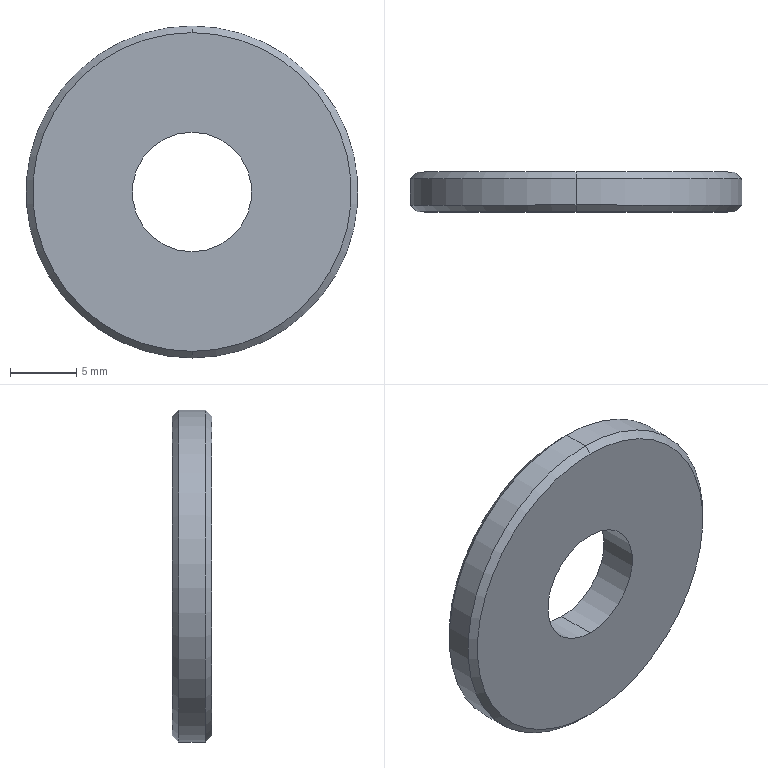Part | SolidWorks | features Chamfer 1, Extrusion 1, ICE 1 | 1 solid | 10 faces | box 25 x 3 x 25 mm | volume 1262 mm3 | cone 4 | cylinder 4 | plane 2 | commonest cylinder face diameters 9 x2 25 x2
STEP:
#1=CARTESIAN_POINT('',(0.,3.,12.));
#2=VERTEX_POINT('',#1);
#3=CARTESIAN_POINT('',(0.,3.,-12.));
#4=VERTEX_POINT('',#3);
#5=CARTESIAN_POINT('',(0.,3.,0.));
#6=DIRECTION('',(0.,1.,0.));
#7=DIRECTION('',(0.,0.,1.));
#8=AXIS2_PLACEMENT_3D('',#5,#6,#7);
#9=CIRCLE('',#8,12.);
#10=EDGE_CURVE('',#2,#4,#9,.T.);
#11=ORIENTED_EDGE('',*,*,#10,.F.);
#12=CARTESIAN_POINT('',(0.,2.5,12.5));
#13=VERTEX_POINT('',#12);
#14=CARTESIAN_POINT('',(0.,3.,12.));
#15=DIRECTION('',(0.,-0.7071,0.7071));
#16=VECTOR('',#15,1000.);
#17=LINE('',#14,#16);
#18=EDGE_CURVE('',#2,#13,#17,.T.);
#19=ORIENTED_EDGE('',*,*,#18,.T.);
#20=CARTESIAN_POINT('',(0.,2.5,-12.5));
#21=VERTEX_POINT('',#20);
#22=CARTESIAN_POINT('',(0.,2.5,0.));
#23=DIRECTION('',(0.,-1.,0.));
#24=DIRECTION('',(0.,0.,1.));
#25=AXIS2_PLACEMENT_3D('',#22,#23,#24);
#26=CIRCLE('',#25,12.5);
#27=EDGE_CURVE('',#21,#13,#26,.T.);
#28=ORIENTED_EDGE('',*,*,#27,.F.);
#29=CARTESIAN_POINT('',(0.,3.,-12.));
#30=DIRECTION('',(0.,-0.7071,-0.7071));
#31=VECTOR('',#30,1000.);
#32=LINE('',#29,#31);
#33=EDGE_CURVE('',#4,#21,#32,.T.);
#34=ORIENTED_EDGE('',*,*,#33,.F.);
#35=EDGE_LOOP('',(#11,#19,#28,#34));
#36=FACE_OUTER_BOUND('',#35,.T.);
#37=CARTESIAN_POINT('',(0.,3.,0.));
#38=DIRECTION('',(0.,-1.,0.));
#39=DIRECTION('',(0.,0.,-1.));
#40=AXIS2_PLACEMENT_3D('',#37,#38,#39);
#41=CONICAL_SURFACE('',#40,12.,0.7854);
#42=ADVANCED_FACE('',(#36),#41,.T.);
#43=CARTESIAN_POINT('',(0.,0.,-12.));
#44=VERTEX_POINT('',#43);
#45=CARTESIAN_POINT('',(0.,0.,12.));
#46=VERTEX_POINT('',#45);
#47=CARTESIAN_POINT('',(0.,0.,0.));
#48=DIRECTION('',(0.,-1.,0.));
#49=DIRECTION('',(0.,0.,1.));
#50=AXIS2_PLACEMENT_3D('',#47,#48,#49);
#51=CIRCLE('',#50,12.);
#52=EDGE_CURVE('',#44,#46,#51,.T.);
#53=ORIENTED_EDGE('',*,*,#52,.F.);
#54=CARTESIAN_POINT('',(0.,0.5,-12.5));
#55=VERTEX_POINT('',#54);
#56=CARTESIAN_POINT('',(0.,0.5,-12.5));
#57=DIRECTION('',(0.,0.7071,-0.7071));
#58=VECTOR('',#57,1000.);
#59=LINE('',#56,#58);
#60=EDGE_CURVE('',#44,#55,#59,.T.);
#61=ORIENTED_EDGE('',*,*,#60,.T.);
#62=CARTESIAN_POINT('',(0.,0.5,12.5));
#63=VERTEX_POINT('',#62);
#64=CARTESIAN_POINT('',(0.,0.5,0.));
#65=DIRECTION('',(0.,1.,0.));
#66=DIRECTION('',(0.,0.,1.));
#67=AXIS2_PLACEMENT_3D('',#64,#65,#66);
#68=CIRCLE('',#67,12.5);
#69=EDGE_CURVE('',#63,#55,#68,.T.);
#70=ORIENTED_EDGE('',*,*,#69,.F.);
#71=CARTESIAN_POINT('',(0.,0.5,12.5));
#72=DIRECTION('',(0.,0.7071,0.7071));
#73=VECTOR('',#72,1000.);
#74=LINE('',#71,#73);
#75=EDGE_CURVE('',#46,#63,#74,.T.);
#76=ORIENTED_EDGE('',*,*,#75,.F.);
#77=EDGE_LOOP('',(#53,#61,#70,#76));
#78=FACE_OUTER_BOUND('',#77,.T.);
#79=CARTESIAN_POINT('',(0.,0.5,0.));
#80=DIRECTION('',(0.,1.,0.));
#81=DIRECTION('',(0.,0.,1.));
#82=AXIS2_PLACEMENT_3D('',#79,#80,#81);
#83=CONICAL_SURFACE('',#82,12.5,0.7854);
#84=ADVANCED_FACE('',(#78),#83,.T.);
#85=CARTESIAN_POINT('',(0.,0.,-4.5));
#86=VERTEX_POINT('',#85);
#87=CARTESIAN_POINT('',(0.,0.,4.5));
#88=VERTEX_POINT('',#87);
#89=CARTESIAN_POINT('',(0.,0.,0.));
#90=DIRECTION('',(0.,1.,0.));
#91=DIRECTION('',(0.,0.,1.));
#92=AXIS2_PLACEMENT_3D('',#89,#90,#91);
#93=CIRCLE('',#92,4.5);
#94=EDGE_CURVE('',#86,#88,#93,.T.);
#95=ORIENTED_EDGE('',*,*,#94,.F.);
#96=CARTESIAN_POINT('',(0.,3.,-4.5));
#97=VERTEX_POINT('',#96);
#98=CARTESIAN_POINT('',(0.,0.,-4.5));
#99=DIRECTION('',(0.,1.,0.));
#100=VECTOR('',#99,1000.);
#101=LINE('',#98,#100);
#102=EDGE_CURVE('',#86,#97,#101,.T.);
#103=ORIENTED_EDGE('',*,*,#102,.T.);
#104=CARTESIAN_POINT('',(0.,3.,4.5));
#105=VERTEX_POINT('',#104);
#106=CARTESIAN_POINT('',(0.,3.,0.));
#107=DIRECTION('',(0.,1.,0.));
#108=DIRECTION('',(0.,0.,1.));
#109=AXIS2_PLACEMENT_3D('',#106,#107,#108);
#110=CIRCLE('',#109,4.5);
#111=EDGE_CURVE('',#97,#105,#110,.T.);
#112=ORIENTED_EDGE('',*,*,#111,.T.);
#113=CARTESIAN_POINT('',(0.,0.,4.5));
#114=DIRECTION('',(0.,1.,0.));
#115=VECTOR('',#114,1000.);
#116=LINE('',#113,#115);
#117=EDGE_CURVE('',#88,#105,#116,.T.);
#118=ORIENTED_EDGE('',*,*,#117,.F.);
#119=EDGE_LOOP('',(#95,#103,#112,#118));
#120=FACE_OUTER_BOUND('',#119,.T.);
#121=CARTESIAN_POINT('',(0.,0.,0.));
#122=DIRECTION('',(0.,1.,0.));
#123=DIRECTION('',(0.,0.,1.));
#124=AXIS2_PLACEMENT_3D('',#121,#122,#123);
#125=CYLINDRICAL_SURFACE('',#124,4.5);
#126=ADVANCED_FACE('',(#120),#125,.F.);
#127=ORIENTED_EDGE('',*,*,#27,.T.);
#128=CARTESIAN_POINT('',(0.,3.,12.5));
#129=DIRECTION('',(0.,-1.,0.));
#130=VECTOR('',#129,1000.);
#131=LINE('',#128,#130);
#132=EDGE_CURVE('',#13,#63,#131,.T.);
#133=ORIENTED_EDGE('',*,*,#132,.T.);
#134=ORIENTED_EDGE('',*,*,#69,.T.);
#135=CARTESIAN_POINT('',(0.,3.,-12.5));
#136=DIRECTION('',(0.,-1.,0.));
#137=VECTOR('',#136,1000.);
#138=LINE('',#135,#137);
#139=EDGE_CURVE('',#21,#55,#138,.T.);
#140=ORIENTED_EDGE('',*,*,#139,.F.);
#141=EDGE_LOOP('',(#127,#133,#134,#140));
#142=FACE_OUTER_BOUND('',#141,.T.);
#143=CARTESIAN_POINT('',(0.,3.,0.));
#144=DIRECTION('',(0.,-1.,0.));
#145=DIRECTION('',(0.,0.,-1.));
#146=AXIS2_PLACEMENT_3D('',#143,#144,#145);
#147=CYLINDRICAL_SURFACE('',#146,12.5);
#148=ADVANCED_FACE('',(#142),#147,.T.);
#149=ORIENTED_EDGE('',*,*,#132,.F.);
#150=CARTESIAN_POINT('',(0.,2.5,0.));
#151=DIRECTION('',(0.,-1.,0.));
#152=DIRECTION('',(0.,0.,1.));
#153=AXIS2_PLACEMENT_3D('',#150,#151,#152);
#154=CIRCLE('',#153,12.5);
#155=EDGE_CURVE('',#13,#21,#154,.T.);
#156=ORIENTED_EDGE('',*,*,#155,.T.);
#157=ORIENTED_EDGE('',*,*,#139,.T.);
#158=CARTESIAN_POINT('',(0.,0.5,0.));
#159=DIRECTION('',(0.,1.,0.));
#160=DIRECTION('',(0.,0.,1.));
#161=AXIS2_PLACEMENT_3D('',#158,#159,#160);
#162=CIRCLE('',#161,12.5);
#163=EDGE_CURVE('',#55,#63,#162,.T.);
#164=ORIENTED_EDGE('',*,*,#163,.T.);
#165=EDGE_LOOP('',(#149,#156,#157,#164));
#166=FACE_OUTER_BOUND('',#165,.T.);
#167=CARTESIAN_POINT('',(0.,3.,0.));
#168=DIRECTION('',(0.,-1.,0.));
#169=DIRECTION('',(0.,0.,-1.));
#170=AXIS2_PLACEMENT_3D('',#167,#168,#169);
#171=CYLINDRICAL_SURFACE('',#170,12.5);
#172=ADVANCED_FACE('',(#166),#171,.T.);
#173=CARTESIAN_POINT('',(0.,3.,0.));
#174=DIRECTION('',(0.,1.,0.));
#175=DIRECTION('',(0.,0.,1.));
#176=AXIS2_PLACEMENT_3D('',#173,#174,#175);
#177=CIRCLE('',#176,12.);
#178=EDGE_CURVE('',#4,#2,#177,.T.);
#179=ORIENTED_EDGE('',*,*,#178,.T.);
#180=ORIENTED_EDGE('',*,*,#10,.T.);
#181=EDGE_LOOP('',(#179,#180));
#182=FACE_OUTER_BOUND('',#181,.T.);
#183=CARTESIAN_POINT('',(0.,3.,0.));
#184=DIRECTION('',(0.,1.,0.));
#185=DIRECTION('',(0.,0.,1.));
#186=AXIS2_PLACEMENT_3D('',#183,#184,#185);
#187=CIRCLE('',#186,4.5);
#188=EDGE_CURVE('',#105,#97,#187,.T.);
#189=ORIENTED_EDGE('',*,*,#188,.F.);
#190=ORIENTED_EDGE('',*,*,#111,.F.);
#191=EDGE_LOOP('',(#189,#190));
#192=FACE_BOUND('',#191,.T.);
#193=CARTESIAN_POINT('',(0.,3.,0.));
#194=DIRECTION('',(0.,1.,0.));
#195=DIRECTION('',(0.,0.,1.));
#196=AXIS2_PLACEMENT_3D('',#193,#194,#195);
#197=PLANE('',#196);
#198=ADVANCED_FACE('',(#182,#192),#197,.T.);
#199=CARTESIAN_POINT('',(0.,0.,0.));
#200=DIRECTION('',(0.,-1.,0.));
#201=DIRECTION('',(0.,0.,1.));
#202=AXIS2_PLACEMENT_3D('',#199,#200,#201);
#203=CIRCLE('',#202,12.);
#204=EDGE_CURVE('',#46,#44,#203,.T.);
#205=ORIENTED_EDGE('',*,*,#204,.T.);
#206=ORIENTED_EDGE('',*,*,#52,.T.);
#207=EDGE_LOOP('',(#205,#206));
#208=FACE_OUTER_BOUND('',#207,.T.);
#209=CARTESIAN_POINT('',(0.,0.,0.));
#210=DIRECTION('',(0.,1.,0.));
#211=DIRECTION('',(0.,0.,1.));
#212=AXIS2_PLACEMENT_3D('',#209,#210,#211);
#213=CIRCLE('',#212,4.5);
#214=EDGE_CURVE('',#88,#86,#213,.T.);
#215=ORIENTED_EDGE('',*,*,#214,.T.);
#216=ORIENTED_EDGE('',*,*,#94,.T.);
#217=EDGE_LOOP('',(#215,#216));
#218=FACE_BOUND('',#217,.T.);
#219=CARTESIAN_POINT('',(0.,0.,0.));
#220=DIRECTION('',(0.,1.,0.));
#221=DIRECTION('',(0.,0.,1.));
#222=AXIS2_PLACEMENT_3D('',#219,#220,#221);
#223=PLANE('',#222);
#224=ADVANCED_FACE('',(#208,#218),#223,.F.);
#225=ORIENTED_EDGE('',*,*,#102,.F.);
#226=ORIENTED_EDGE('',*,*,#214,.F.);
#227=ORIENTED_EDGE('',*,*,#117,.T.);
#228=ORIENTED_EDGE('',*,*,#188,.T.);
#229=EDGE_LOOP('',(#225,#226,#227,#228));
#230=FACE_OUTER_BOUND('',#229,.T.);
#231=CARTESIAN_POINT('',(0.,0.,0.));
#232=DIRECTION('',(0.,1.,0.));
#233=DIRECTION('',(0.,0.,1.));
#234=AXIS2_PLACEMENT_3D('',#231,#232,#233);
#235=CYLINDRICAL_SURFACE('',#234,4.5);
#236=ADVANCED_FACE('',(#230),#235,.F.);
#237=ORIENTED_EDGE('',*,*,#60,.F.);
#238=ORIENTED_EDGE('',*,*,#204,.F.);
#239=ORIENTED_EDGE('',*,*,#75,.T.);
#240=ORIENTED_EDGE('',*,*,#163,.F.);
#241=EDGE_LOOP('',(#237,#238,#239,#240));
#242=FACE_OUTER_BOUND('',#241,.T.);
#243=CARTESIAN_POINT('',(0.,0.5,0.));
#244=DIRECTION('',(0.,1.,0.));
#245=DIRECTION('',(0.,0.,1.));
#246=AXIS2_PLACEMENT_3D('',#243,#244,#245);
#247=CONICAL_SURFACE('',#246,12.5,0.7854);
#248=ADVANCED_FACE('',(#242),#247,.T.);
#249=ORIENTED_EDGE('',*,*,#18,.F.);
#250=ORIENTED_EDGE('',*,*,#178,.F.);
#251=ORIENTED_EDGE('',*,*,#33,.T.);
#252=ORIENTED_EDGE('',*,*,#155,.F.);
#253=EDGE_LOOP('',(#249,#250,#251,#252));
#254=FACE_OUTER_BOUND('',#253,.T.);
#255=CARTESIAN_POINT('',(0.,3.,0.));
#256=DIRECTION('',(0.,-1.,0.));
#257=DIRECTION('',(0.,0.,-1.));
#258=AXIS2_PLACEMENT_3D('',#255,#256,#257);
#259=CONICAL_SURFACE('',#258,12.,0.7854);
#260=ADVANCED_FACE('',(#254),#259,.T.);
#261=CLOSED_SHELL('',(#42,#84,#126,#148,#172,#198,#224,#236,#248,#260));
#262=MANIFOLD_SOLID_BREP('',#261);
#263=CARTESIAN_POINT('',(0.,0.,0.));
#264=DIRECTION('',(0.,0.,1.));
#265=DIRECTION('',(1.,0.,0.));
#266=AXIS2_PLACEMENT_3D('',#263,#264,#265);
#267=(LENGTH_UNIT()NAMED_UNIT(*)SI_UNIT(.MILLI.,.METRE.));
#268=UNCERTAINTY_MEASURE_WITH_UNIT(LENGTH_MEASURE(0.00001),#267,'','');
#269=(NAMED_UNIT(*)PLANE_ANGLE_UNIT()SI_UNIT($,.RADIAN.));
#270=(NAMED_UNIT(*)SI_UNIT($,.STERADIAN.)SOLID_ANGLE_UNIT());
#271=(GEOMETRIC_REPRESENTATION_CONTEXT(3)GLOBAL_UNCERTAINTY_ASSIGNED_CONTEXT((#268))GLOBAL_UNIT_ASSIGNED_CONTEXT((#267,#269,#270))REPRESENTATION_CONTEXT('',''));
#272=ADVANCED_BREP_SHAPE_REPRESENTATION('',(#262,#266),#271);